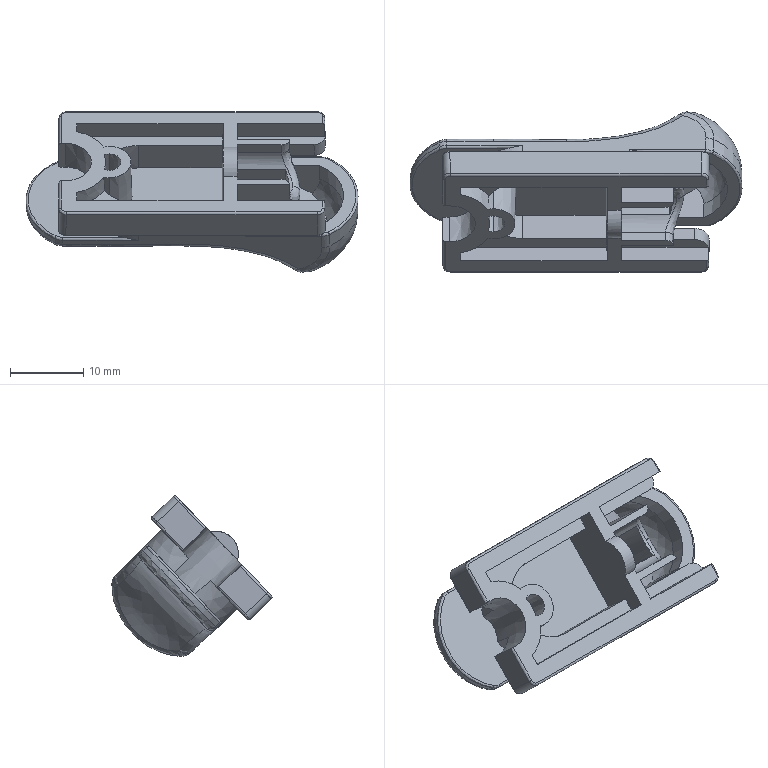Part | SolidWorks | features BaseBody 1 | 1 solid | 131 faces | box 45.446 x 21.894 x 21.945 mm | volume 4020 mm3 | spline 42 | plane 42 | cylinder 29 | cone 18 | commonest cylinder face diameters 0.6 x16 2 x4 55.3 x2 3 x1 4 x1 6.2 x1